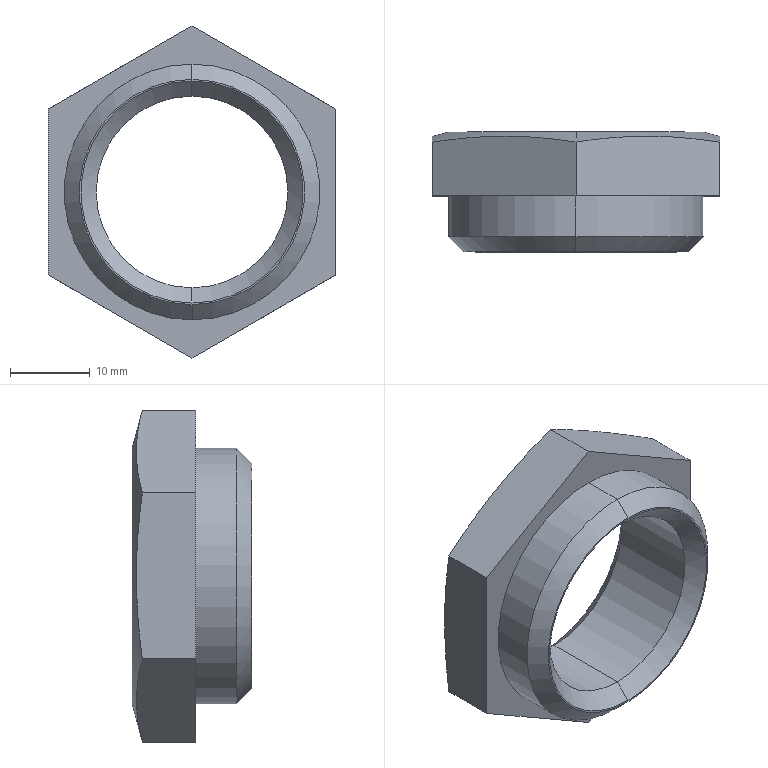Part | SolidWorks | features Boss 1, RevCut 1, Revolution 1 | 1 solid | 21 faces | box 36 x 15 x 41.569 mm | volume 7224 mm3 | plane 9 | cone 8 | cylinder 4 | commonest cylinder face diameters 24 x2 32 x2
STEP:
#1=CARTESIAN_POINT('',(0.,13.1,-12.));
#2=VERTEX_POINT('',#1);
#3=CARTESIAN_POINT('',(0.,13.1,12.));
#4=VERTEX_POINT('',#3);
#5=CARTESIAN_POINT('',(0.,13.1,0.));
#6=DIRECTION('',(0.,1.,0.));
#7=DIRECTION('',(0.,0.,1.));
#8=AXIS2_PLACEMENT_3D('',#5,#6,#7);
#9=CIRCLE('',#8,12.);
#10=EDGE_CURVE('',#2,#4,#9,.T.);
#11=ORIENTED_EDGE('',*,*,#10,.F.);
#12=CARTESIAN_POINT('',(0.,15.,-13.9));
#13=VERTEX_POINT('',#12);
#14=CARTESIAN_POINT('',(0.,15.,-13.9));
#15=DIRECTION('',(0.,0.7071,-0.7071));
#16=VECTOR('',#15,1000.);
#17=LINE('',#14,#16);
#18=EDGE_CURVE('',#2,#13,#17,.T.);
#19=ORIENTED_EDGE('',*,*,#18,.T.);
#20=CARTESIAN_POINT('',(0.,15.,13.9));
#21=VERTEX_POINT('',#20);
#22=CARTESIAN_POINT('',(0.,15.,0.));
#23=DIRECTION('',(0.,1.,0.));
#24=DIRECTION('',(0.,0.,1.));
#25=AXIS2_PLACEMENT_3D('',#22,#23,#24);
#26=CIRCLE('',#25,13.9);
#27=EDGE_CURVE('',#13,#21,#26,.T.);
#28=ORIENTED_EDGE('',*,*,#27,.T.);
#29=CARTESIAN_POINT('',(0.,15.,13.9));
#30=DIRECTION('',(0.,0.7071,0.7071));
#31=VECTOR('',#30,1000.);
#32=LINE('',#29,#31);
#33=EDGE_CURVE('',#4,#21,#32,.T.);
#34=ORIENTED_EDGE('',*,*,#33,.F.);
#35=EDGE_LOOP('',(#11,#19,#28,#34));
#36=FACE_OUTER_BOUND('',#35,.T.);
#37=CARTESIAN_POINT('',(0.,15.,0.));
#38=DIRECTION('',(0.,1.,0.));
#39=DIRECTION('',(0.,0.,1.));
#40=AXIS2_PLACEMENT_3D('',#37,#38,#39);
#41=CONICAL_SURFACE('',#40,13.9,0.7854);
#42=ADVANCED_FACE('',(#36),#41,.F.);
#43=CARTESIAN_POINT('',(0.,15.,16.));
#44=VERTEX_POINT('',#43);
#45=CARTESIAN_POINT('',(0.,15.,-16.));
#46=VERTEX_POINT('',#45);
#47=CARTESIAN_POINT('',(0.,15.,0.));
#48=DIRECTION('',(0.,1.,0.));
#49=DIRECTION('',(0.,0.,1.));
#50=AXIS2_PLACEMENT_3D('',#47,#48,#49);
#51=CIRCLE('',#50,16.);
#52=EDGE_CURVE('',#44,#46,#51,.T.);
#53=ORIENTED_EDGE('',*,*,#52,.F.);
#54=CARTESIAN_POINT('',(0.,13.718,20.785));
#55=VERTEX_POINT('',#54);
#56=CARTESIAN_POINT('',(0.,11.276,29.9));
#57=DIRECTION('',(0.,-0.2588,0.9659));
#58=VECTOR('',#57,1000.);
#59=LINE('',#56,#58);
#60=EDGE_CURVE('',#44,#55,#59,.T.);
#61=ORIENTED_EDGE('',*,*,#60,.T.);
#62=CARTESIAN_POINT('',(18.,13.718,10.392));
#63=VERTEX_POINT('',#62);
#64=CARTESIAN_POINT('',(0.,13.718,20.785));
#65=CARTESIAN_POINT('',(1.5,13.95,19.919));
#66=CARTESIAN_POINT('',(3.,14.138,19.053));
#67=CARTESIAN_POINT('',(6.,14.396,17.321));
#68=CARTESIAN_POINT('',(9.,14.532,15.588));
#69=CARTESIAN_POINT('',(12.,14.396,13.856));
#70=CARTESIAN_POINT('',(15.,14.138,12.124));
#71=CARTESIAN_POINT('',(16.5,13.95,11.258));
#72=CARTESIAN_POINT('',(18.,13.718,10.392));
#73=B_SPLINE_CURVE_WITH_KNOTS('',3,(#64,#65,#66,#67,#68,#69,#70,#71,#72),.UNSPECIFIED.,.F.,.F.,(4,2,1,2,4),(0.000000231,0.005196,0.01039,0.01559,0.02078),.UNSPECIFIED.);
#74=EDGE_CURVE('',#55,#63,#73,.T.);
#75=ORIENTED_EDGE('',*,*,#74,.T.);
#76=CARTESIAN_POINT('',(18.,13.718,-10.392));
#77=VERTEX_POINT('',#76);
#78=CARTESIAN_POINT('',(18.,13.718,10.392));
#79=CARTESIAN_POINT('',(18.,13.949,8.666));
#80=CARTESIAN_POINT('',(18.,14.137,6.939));
#81=CARTESIAN_POINT('',(18.,14.395,3.481));
#82=CARTESIAN_POINT('',(18.,14.464,1.75));
#83=CARTESIAN_POINT('',(18.,14.465,-1.715));
#84=CARTESIAN_POINT('',(18.,14.397,-3.449));
#85=CARTESIAN_POINT('',(18.,14.139,-6.922));
#86=CARTESIAN_POINT('',(18.,13.95,-8.662));
#87=CARTESIAN_POINT('',(18.,13.718,-10.392));
#88=B_SPLINE_CURVE_WITH_KNOTS('',3,(#78,#79,#80,#81,#82,#83,#84,#85,#86,#87),.UNSPECIFIED.,.F.,.F.,(4,2,2,2,4),(0.04105,0.04627,0.05149,0.05671,0.06193),.UNSPECIFIED.);
#89=EDGE_CURVE('',#63,#77,#88,.T.);
#90=ORIENTED_EDGE('',*,*,#89,.T.);
#91=CARTESIAN_POINT('',(0.,13.718,-20.785));
#92=VERTEX_POINT('',#91);
#93=CARTESIAN_POINT('',(18.,13.718,-10.392));
#94=CARTESIAN_POINT('',(16.5,13.95,-11.258));
#95=CARTESIAN_POINT('',(15.,14.138,-12.124));
#96=CARTESIAN_POINT('',(12.,14.396,-13.856));
#97=CARTESIAN_POINT('',(9.,14.532,-15.588));
#98=CARTESIAN_POINT('',(6.,14.396,-17.321));
#99=CARTESIAN_POINT('',(3.,14.138,-19.053));
#100=CARTESIAN_POINT('',(1.5,13.95,-19.919));
#101=CARTESIAN_POINT('',(0.,13.718,-20.785));
#102=B_SPLINE_CURVE_WITH_KNOTS('',3,(#93,#94,#95,#96,#97,#98,#99,#100,#101),.UNSPECIFIED.,.F.,.F.,(4,2,1,2,4),(0.000000231,0.005196,0.01039,0.01559,0.02078),.UNSPECIFIED.);
#103=EDGE_CURVE('',#77,#92,#102,.T.);
#104=ORIENTED_EDGE('',*,*,#103,.T.);
#105=CARTESIAN_POINT('',(0.,11.276,-29.9));
#106=DIRECTION('',(0.,-0.2588,-0.9659));
#107=VECTOR('',#106,1000.);
#108=LINE('',#105,#107);
#109=EDGE_CURVE('',#46,#92,#108,.T.);
#110=ORIENTED_EDGE('',*,*,#109,.F.);
#111=EDGE_LOOP('',(#53,#61,#75,#90,#104,#110));
#112=FACE_OUTER_BOUND('',#111,.T.);
#113=CARTESIAN_POINT('',(0.,11.276,0.));
#114=DIRECTION('',(0.,-1.,0.));
#115=DIRECTION('',(0.,0.,-1.));
#116=AXIS2_PLACEMENT_3D('',#113,#114,#115);
#117=CONICAL_SURFACE('',#116,29.9,1.309);
#118=ADVANCED_FACE('',(#112),#117,.T.);
#119=CARTESIAN_POINT('',(0.,1.9,-12.));
#120=VERTEX_POINT('',#119);
#121=CARTESIAN_POINT('',(0.,1.9,12.));
#122=VERTEX_POINT('',#121);
#123=CARTESIAN_POINT('',(0.,1.9,0.));
#124=DIRECTION('',(0.,1.,0.));
#125=DIRECTION('',(0.,0.,1.));
#126=AXIS2_PLACEMENT_3D('',#123,#124,#125);
#127=CIRCLE('',#126,12.);
#128=EDGE_CURVE('',#120,#122,#127,.T.);
#129=ORIENTED_EDGE('',*,*,#128,.F.);
#130=CARTESIAN_POINT('',(0.,0.,-12.));
#131=DIRECTION('',(0.,1.,0.));
#132=VECTOR('',#131,1000.);
#133=LINE('',#130,#132);
#134=EDGE_CURVE('',#120,#2,#133,.T.);
#135=ORIENTED_EDGE('',*,*,#134,.T.);
#136=ORIENTED_EDGE('',*,*,#10,.T.);
#137=CARTESIAN_POINT('',(0.,0.,12.));
#138=DIRECTION('',(0.,1.,0.));
#139=VECTOR('',#138,1000.);
#140=LINE('',#137,#139);
#141=EDGE_CURVE('',#122,#4,#140,.T.);
#142=ORIENTED_EDGE('',*,*,#141,.F.);
#143=EDGE_LOOP('',(#129,#135,#136,#142));
#144=FACE_OUTER_BOUND('',#143,.T.);
#145=CARTESIAN_POINT('',(0.,0.,0.));
#146=DIRECTION('',(0.,1.,0.));
#147=DIRECTION('',(0.,0.,1.));
#148=AXIS2_PLACEMENT_3D('',#145,#146,#147);
#149=CYLINDRICAL_SURFACE('',#148,12.);
#150=ADVANCED_FACE('',(#144),#149,.F.);
#151=CARTESIAN_POINT('',(0.,1.9,16.));
#152=VERTEX_POINT('',#151);
#153=CARTESIAN_POINT('',(0.,1.9,-16.));
#154=VERTEX_POINT('',#153);
#155=CARTESIAN_POINT('',(0.,1.9,0.));
#156=DIRECTION('',(0.,1.,0.));
#157=DIRECTION('',(0.,0.,1.));
#158=AXIS2_PLACEMENT_3D('',#155,#156,#157);
#159=CIRCLE('',#158,16.);
#160=EDGE_CURVE('',#152,#154,#159,.T.);
#161=ORIENTED_EDGE('',*,*,#160,.T.);
#162=CARTESIAN_POINT('',(0.,7.,-16.));
#163=VERTEX_POINT('',#162);
#164=CARTESIAN_POINT('',(0.,0.,-16.));
#165=DIRECTION('',(0.,1.,0.));
#166=VECTOR('',#165,1000.);
#167=LINE('',#164,#166);
#168=EDGE_CURVE('',#154,#163,#167,.T.);
#169=ORIENTED_EDGE('',*,*,#168,.T.);
#170=CARTESIAN_POINT('',(0.,7.,16.));
#171=VERTEX_POINT('',#170);
#172=CARTESIAN_POINT('',(0.,7.,0.));
#173=DIRECTION('',(0.,1.,0.));
#174=DIRECTION('',(0.,0.,1.));
#175=AXIS2_PLACEMENT_3D('',#172,#173,#174);
#176=CIRCLE('',#175,16.);
#177=EDGE_CURVE('',#171,#163,#176,.T.);
#178=ORIENTED_EDGE('',*,*,#177,.F.);
#179=CARTESIAN_POINT('',(0.,0.,16.));
#180=DIRECTION('',(0.,1.,0.));
#181=VECTOR('',#180,1000.);
#182=LINE('',#179,#181);
#183=EDGE_CURVE('',#152,#171,#182,.T.);
#184=ORIENTED_EDGE('',*,*,#183,.F.);
#185=EDGE_LOOP('',(#161,#169,#178,#184));
#186=FACE_OUTER_BOUND('',#185,.T.);
#187=CARTESIAN_POINT('',(0.,0.,0.));
#188=DIRECTION('',(0.,1.,0.));
#189=DIRECTION('',(0.,0.,1.));
#190=AXIS2_PLACEMENT_3D('',#187,#188,#189);
#191=CYLINDRICAL_SURFACE('',#190,16.);
#192=ADVANCED_FACE('',(#186),#191,.T.);
#193=CARTESIAN_POINT('',(0.,0.,14.1));
#194=VERTEX_POINT('',#193);
#195=CARTESIAN_POINT('',(0.,0.,-14.1));
#196=VERTEX_POINT('',#195);
#197=CARTESIAN_POINT('',(0.,0.,0.));
#198=DIRECTION('',(0.,1.,0.));
#199=DIRECTION('',(0.,0.,1.));
#200=AXIS2_PLACEMENT_3D('',#197,#198,#199);
#201=CIRCLE('',#200,14.1);
#202=EDGE_CURVE('',#194,#196,#201,.T.);
#203=ORIENTED_EDGE('',*,*,#202,.T.);
#204=CARTESIAN_POINT('',(0.,1.9,-16.));
#205=DIRECTION('',(0.,0.7071,-0.7071));
#206=VECTOR('',#205,1000.);
#207=LINE('',#204,#206);
#208=EDGE_CURVE('',#196,#154,#207,.T.);
#209=ORIENTED_EDGE('',*,*,#208,.T.);
#210=ORIENTED_EDGE('',*,*,#160,.F.);
#211=CARTESIAN_POINT('',(0.,1.9,16.));
#212=DIRECTION('',(0.,0.7071,0.7071));
#213=VECTOR('',#212,1000.);
#214=LINE('',#211,#213);
#215=EDGE_CURVE('',#194,#152,#214,.T.);
#216=ORIENTED_EDGE('',*,*,#215,.F.);
#217=EDGE_LOOP('',(#203,#209,#210,#216));
#218=FACE_OUTER_BOUND('',#217,.T.);
#219=CARTESIAN_POINT('',(0.,1.9,0.));
#220=DIRECTION('',(0.,1.,0.));
#221=DIRECTION('',(0.,0.,1.));
#222=AXIS2_PLACEMENT_3D('',#219,#220,#221);
#223=CONICAL_SURFACE('',#222,16.,0.7854);
#224=ADVANCED_FACE('',(#218),#223,.T.);
#225=ORIENTED_EDGE('',*,*,#128,.T.);
#226=CARTESIAN_POINT('',(0.,0.,13.9));
#227=VERTEX_POINT('',#226);
#228=CARTESIAN_POINT('',(0.,0.,13.9));
#229=DIRECTION('',(0.,-0.7071,0.7071));
#230=VECTOR('',#229,1000.);
#231=LINE('',#228,#230);
#232=EDGE_CURVE('',#122,#227,#231,.T.);
#233=ORIENTED_EDGE('',*,*,#232,.T.);
#234=CARTESIAN_POINT('',(0.,0.,-13.9));
#235=VERTEX_POINT('',#234);
#236=CARTESIAN_POINT('',(0.,0.,0.));
#237=DIRECTION('',(0.,1.,0.));
#238=DIRECTION('',(0.,0.,1.));
#239=AXIS2_PLACEMENT_3D('',#236,#237,#238);
#240=CIRCLE('',#239,13.9);
#241=EDGE_CURVE('',#235,#227,#240,.T.);
#242=ORIENTED_EDGE('',*,*,#241,.F.);
#243=CARTESIAN_POINT('',(0.,0.,-13.9));
#244=DIRECTION('',(0.,-0.7071,-0.7071));
#245=VECTOR('',#244,1000.);
#246=LINE('',#243,#245);
#247=EDGE_CURVE('',#120,#235,#246,.T.);
#248=ORIENTED_EDGE('',*,*,#247,.F.);
#249=EDGE_LOOP('',(#225,#233,#242,#248));
#250=FACE_OUTER_BOUND('',#249,.T.);
#251=CARTESIAN_POINT('',(0.,0.,0.));
#252=DIRECTION('',(0.,-1.,0.));
#253=DIRECTION('',(0.,0.,-1.));
#254=AXIS2_PLACEMENT_3D('',#251,#252,#253);
#255=CONICAL_SURFACE('',#254,13.9,0.7854);
#256=ADVANCED_FACE('',(#250),#255,.F.);
#257=ORIENTED_EDGE('',*,*,#232,.F.);
#258=CARTESIAN_POINT('',(0.,1.9,0.));
#259=DIRECTION('',(0.,1.,0.));
#260=DIRECTION('',(0.,0.,1.));
#261=AXIS2_PLACEMENT_3D('',#258,#259,#260);
#262=CIRCLE('',#261,12.);
#263=EDGE_CURVE('',#122,#120,#262,.T.);
#264=ORIENTED_EDGE('',*,*,#263,.T.);
#265=ORIENTED_EDGE('',*,*,#247,.T.);
#266=CARTESIAN_POINT('',(0.,0.,0.));
#267=DIRECTION('',(0.,1.,0.));
#268=DIRECTION('',(0.,0.,1.));
#269=AXIS2_PLACEMENT_3D('',#266,#267,#268);
#270=CIRCLE('',#269,13.9);
#271=EDGE_CURVE('',#227,#235,#270,.T.);
#272=ORIENTED_EDGE('',*,*,#271,.F.);
#273=EDGE_LOOP('',(#257,#264,#265,#272));
#274=FACE_OUTER_BOUND('',#273,.T.);
#275=CARTESIAN_POINT('',(0.,0.,0.));
#276=DIRECTION('',(0.,-1.,0.));
#277=DIRECTION('',(0.,0.,-1.));
#278=AXIS2_PLACEMENT_3D('',#275,#276,#277);
#279=CONICAL_SURFACE('',#278,13.9,0.7854);
#280=ADVANCED_FACE('',(#274),#279,.F.);
#281=ORIENTED_EDGE('',*,*,#241,.T.);
#282=ORIENTED_EDGE('',*,*,#271,.T.);
#283=EDGE_LOOP('',(#281,#282));
#284=FACE_BOUND('',#283,.T.);
#285=ORIENTED_EDGE('',*,*,#202,.F.);
#286=CARTESIAN_POINT('',(0.,0.,0.));
#287=DIRECTION('',(0.,1.,0.));
#288=DIRECTION('',(0.,0.,1.));
#289=AXIS2_PLACEMENT_3D('',#286,#287,#288);
#290=CIRCLE('',#289,14.1);
#291=EDGE_CURVE('',#196,#194,#290,.T.);
#292=ORIENTED_EDGE('',*,*,#291,.F.);
#293=EDGE_LOOP('',(#285,#292));
#294=FACE_OUTER_BOUND('',#293,.T.);
#295=CARTESIAN_POINT('',(-13.9,0.,0.));
#296=DIRECTION('',(0.,-1.,0.));
#297=DIRECTION('',(0.,0.,-1.));
#298=AXIS2_PLACEMENT_3D('',#295,#296,#297);
#299=PLANE('',#298);
#300=ADVANCED_FACE('',(#284,#294),#299,.T.);
#301=ORIENTED_EDGE('',*,*,#208,.F.);
#302=ORIENTED_EDGE('',*,*,#291,.T.);
#303=ORIENTED_EDGE('',*,*,#215,.T.);
#304=CARTESIAN_POINT('',(0.,1.9,0.));
#305=DIRECTION('',(0.,1.,0.));
#306=DIRECTION('',(0.,0.,1.));
#307=AXIS2_PLACEMENT_3D('',#304,#305,#306);
#308=CIRCLE('',#307,16.);
#309=EDGE_CURVE('',#154,#152,#308,.T.);
#310=ORIENTED_EDGE('',*,*,#309,.F.);
#311=EDGE_LOOP('',(#301,#302,#303,#310));
#312=FACE_OUTER_BOUND('',#311,.T.);
#313=CARTESIAN_POINT('',(0.,1.9,0.));
#314=DIRECTION('',(0.,1.,0.));
#315=DIRECTION('',(0.,0.,1.));
#316=AXIS2_PLACEMENT_3D('',#313,#314,#315);
#317=CONICAL_SURFACE('',#316,16.,0.7854);
#318=ADVANCED_FACE('',(#312),#317,.T.);
#319=ORIENTED_EDGE('',*,*,#168,.F.);
#320=ORIENTED_EDGE('',*,*,#309,.T.);
#321=ORIENTED_EDGE('',*,*,#183,.T.);
#322=CARTESIAN_POINT('',(0.,7.,0.));
#323=DIRECTION('',(0.,1.,0.));
#324=DIRECTION('',(0.,0.,1.));
#325=AXIS2_PLACEMENT_3D('',#322,#323,#324);
#326=CIRCLE('',#325,16.);
#327=EDGE_CURVE('',#163,#171,#326,.T.);
#328=ORIENTED_EDGE('',*,*,#327,.F.);
#329=EDGE_LOOP('',(#319,#320,#321,#328));
#330=FACE_OUTER_BOUND('',#329,.T.);
#331=CARTESIAN_POINT('',(0.,0.,0.));
#332=DIRECTION('',(0.,1.,0.));
#333=DIRECTION('',(0.,0.,1.));
#334=AXIS2_PLACEMENT_3D('',#331,#332,#333);
#335=CYLINDRICAL_SURFACE('',#334,16.);
#336=ADVANCED_FACE('',(#330),#335,.T.);
#337=ORIENTED_EDGE('',*,*,#177,.T.);
#338=ORIENTED_EDGE('',*,*,#327,.T.);
#339=EDGE_LOOP('',(#337,#338));
#340=FACE_BOUND('',#339,.T.);
#341=CARTESIAN_POINT('',(18.,7.,10.392));
#342=VERTEX_POINT('',#341);
#343=CARTESIAN_POINT('',(18.,7.,-10.392));
#344=VERTEX_POINT('',#343);
#345=CARTESIAN_POINT('',(18.,7.,10.392));
#346=DIRECTION('',(0.,0.,-1.));
#347=VECTOR('',#346,1000.);
#348=LINE('',#345,#347);
#349=EDGE_CURVE('',#342,#344,#348,.T.);
#350=ORIENTED_EDGE('',*,*,#349,.F.);
#351=CARTESIAN_POINT('',(0.,7.,20.785));
#352=VERTEX_POINT('',#351);
#353=CARTESIAN_POINT('',(0.,7.,20.785));
#354=DIRECTION('',(0.866,0.,-0.5));
#355=VECTOR('',#354,1000.);
#356=LINE('',#353,#355);
#357=EDGE_CURVE('',#352,#342,#356,.T.);
#358=ORIENTED_EDGE('',*,*,#357,.F.);
#359=CARTESIAN_POINT('',(-18.,7.,10.392));
#360=VERTEX_POINT('',#359);
#361=CARTESIAN_POINT('',(-18.,7.,10.392));
#362=DIRECTION('',(0.866,0.,0.5));
#363=VECTOR('',#362,1000.);
#364=LINE('',#361,#363);
#365=EDGE_CURVE('',#360,#352,#364,.T.);
#366=ORIENTED_EDGE('',*,*,#365,.F.);
#367=CARTESIAN_POINT('',(-18.,7.,-10.392));
#368=VERTEX_POINT('',#367);
#369=CARTESIAN_POINT('',(-18.,7.,-10.392));
#370=DIRECTION('',(0.,0.,1.));
#371=VECTOR('',#370,1000.);
#372=LINE('',#369,#371);
#373=EDGE_CURVE('',#368,#360,#372,.T.);
#374=ORIENTED_EDGE('',*,*,#373,.F.);
#375=CARTESIAN_POINT('',(0.,7.,-20.785));
#376=VERTEX_POINT('',#375);
#377=CARTESIAN_POINT('',(0.,7.,-20.785));
#378=DIRECTION('',(-0.866,0.,0.5));
#379=VECTOR('',#378,1000.);
#380=LINE('',#377,#379);
#381=EDGE_CURVE('',#376,#368,#380,.T.);
#382=ORIENTED_EDGE('',*,*,#381,.F.);
#383=CARTESIAN_POINT('',(18.,7.,-10.392));
#384=DIRECTION('',(-0.866,0.,-0.5));
#385=VECTOR('',#384,1000.);
#386=LINE('',#383,#385);
#387=EDGE_CURVE('',#344,#376,#386,.T.);
#388=ORIENTED_EDGE('',*,*,#387,.F.);
#389=EDGE_LOOP('',(#350,#358,#366,#374,#382,#388));
#390=FACE_OUTER_BOUND('',#389,.T.);
#391=CARTESIAN_POINT('',(-16.,7.,0.));
#392=DIRECTION('',(0.,-1.,0.));
#393=DIRECTION('',(0.,0.,-1.));
#394=AXIS2_PLACEMENT_3D('',#391,#392,#393);
#395=PLANE('',#394);
#396=ADVANCED_FACE('',(#340,#390),#395,.T.);
#397=ORIENTED_EDGE('',*,*,#134,.F.);
#398=ORIENTED_EDGE('',*,*,#263,.F.);
#399=ORIENTED_EDGE('',*,*,#141,.T.);
#400=CARTESIAN_POINT('',(0.,13.1,0.));
#401=DIRECTION('',(0.,1.,0.));
#402=DIRECTION('',(0.,0.,1.));
#403=AXIS2_PLACEMENT_3D('',#400,#401,#402);
#404=CIRCLE('',#403,12.);
#405=EDGE_CURVE('',#4,#2,#404,.T.);
#406=ORIENTED_EDGE('',*,*,#405,.T.);
#407=EDGE_LOOP('',(#397,#398,#399,#406));
#408=FACE_OUTER_BOUND('',#407,.T.);
#409=CARTESIAN_POINT('',(0.,0.,0.));
#410=DIRECTION('',(0.,1.,0.));
#411=DIRECTION('',(0.,0.,1.));
#412=AXIS2_PLACEMENT_3D('',#409,#410,#411);
#413=CYLINDRICAL_SURFACE('',#412,12.);
#414=ADVANCED_FACE('',(#408),#413,.F.);
#415=ORIENTED_EDGE('',*,*,#74,.F.);
#416=CARTESIAN_POINT('',(0.,7.,20.785));
#417=DIRECTION('',(0.,1.,0.));
#418=VECTOR('',#417,1000.);
#419=LINE('',#416,#418);
#420=EDGE_CURVE('',#352,#55,#419,.T.);
#421=ORIENTED_EDGE('',*,*,#420,.F.);
#422=ORIENTED_EDGE('',*,*,#357,.T.);
#423=CARTESIAN_POINT('',(18.,7.,10.392));
#424=DIRECTION('',(0.,1.,0.));
#425=VECTOR('',#424,1000.);
#426=LINE('',#423,#425);
#427=EDGE_CURVE('',#342,#63,#426,.T.);
#428=ORIENTED_EDGE('',*,*,#427,.T.);
#429=EDGE_LOOP('',(#415,#421,#422,#428));
#430=FACE_OUTER_BOUND('',#429,.T.);
#431=CARTESIAN_POINT('',(0.,7.,20.785));
#432=DIRECTION('',(0.5,0.,0.866));
#433=DIRECTION('',(0.866,0.,-0.5));
#434=AXIS2_PLACEMENT_3D('',#431,#432,#433);
#435=PLANE('',#434);
#436=ADVANCED_FACE('',(#430),#435,.T.);
#437=CARTESIAN_POINT('',(-18.,13.718,10.392));
#438=VERTEX_POINT('',#437);
#439=CARTESIAN_POINT('',(-18.,13.718,10.392));
#440=CARTESIAN_POINT('',(-16.5,13.95,11.258));
#441=CARTESIAN_POINT('',(-15.,14.138,12.124));
#442=CARTESIAN_POINT('',(-12.,14.396,13.856));
#443=CARTESIAN_POINT('',(-9.,14.532,15.588));
#444=CARTESIAN_POINT('',(-6.,14.396,17.321));
#445=CARTESIAN_POINT('',(-3.,14.138,19.053));
#446=CARTESIAN_POINT('',(-1.5,13.95,19.919));
#447=CARTESIAN_POINT('',(0.,13.718,20.785));
#448=B_SPLINE_CURVE_WITH_KNOTS('',3,(#439,#440,#441,#442,#443,#444,#445,#446,#447),.UNSPECIFIED.,.F.,.F.,(4,2,1,2,4),(0.000000231,0.005196,0.01039,0.01559,0.02078),.UNSPECIFIED.);
#449=EDGE_CURVE('',#438,#55,#448,.T.);
#450=ORIENTED_EDGE('',*,*,#449,.F.);
#451=CARTESIAN_POINT('',(-18.,7.,10.392));
#452=DIRECTION('',(0.,1.,0.));
#453=VECTOR('',#452,1000.);
#454=LINE('',#451,#453);
#455=EDGE_CURVE('',#360,#438,#454,.T.);
#456=ORIENTED_EDGE('',*,*,#455,.F.);
#457=ORIENTED_EDGE('',*,*,#365,.T.);
#458=ORIENTED_EDGE('',*,*,#420,.T.);
#459=EDGE_LOOP('',(#450,#456,#457,#458));
#460=FACE_OUTER_BOUND('',#459,.T.);
#461=CARTESIAN_POINT('',(-18.,7.,10.392));
#462=DIRECTION('',(-0.5,0.,0.866));
#463=DIRECTION('',(0.866,0.,0.5));
#464=AXIS2_PLACEMENT_3D('',#461,#462,#463);
#465=PLANE('',#464);
#466=ADVANCED_FACE('',(#460),#465,.T.);
#467=CARTESIAN_POINT('',(-18.,13.718,-10.392));
#468=VERTEX_POINT('',#467);
#469=CARTESIAN_POINT('',(-18.,13.718,-10.392));
#470=CARTESIAN_POINT('',(-18.,13.95,-8.662));
#471=CARTESIAN_POINT('',(-18.,14.139,-6.922));
#472=CARTESIAN_POINT('',(-18.,14.397,-3.449));
#473=CARTESIAN_POINT('',(-18.,14.465,-1.715));
#474=CARTESIAN_POINT('',(-18.,14.464,1.75));
#475=CARTESIAN_POINT('',(-18.,14.395,3.481));
#476=CARTESIAN_POINT('',(-18.,14.137,6.939));
#477=CARTESIAN_POINT('',(-18.,13.949,8.666));
#478=CARTESIAN_POINT('',(-18.,13.718,10.392));
#479=B_SPLINE_CURVE_WITH_KNOTS('',3,(#469,#470,#471,#472,#473,#474,#475,#476,#477,#478),.UNSPECIFIED.,.F.,.F.,(4,2,2,2,4),(0.01753,0.02276,0.02799,0.03322,0.03845),.UNSPECIFIED.);
#480=EDGE_CURVE('',#468,#438,#479,.T.);
#481=ORIENTED_EDGE('',*,*,#480,.F.);
#482=CARTESIAN_POINT('',(-18.,7.,-10.392));
#483=DIRECTION('',(0.,1.,0.));
#484=VECTOR('',#483,1000.);
#485=LINE('',#482,#484);
#486=EDGE_CURVE('',#368,#468,#485,.T.);
#487=ORIENTED_EDGE('',*,*,#486,.F.);
#488=ORIENTED_EDGE('',*,*,#373,.T.);
#489=ORIENTED_EDGE('',*,*,#455,.T.);
#490=EDGE_LOOP('',(#481,#487,#488,#489));
#491=FACE_OUTER_BOUND('',#490,.T.);
#492=CARTESIAN_POINT('',(-18.,7.,-10.392));
#493=DIRECTION('',(-1.,0.,0.));
#494=DIRECTION('',(0.,0.,1.));
#495=AXIS2_PLACEMENT_3D('',#492,#493,#494);
#496=PLANE('',#495);
#497=ADVANCED_FACE('',(#491),#496,.T.);
#498=CARTESIAN_POINT('',(0.,13.718,-20.785));
#499=CARTESIAN_POINT('',(-1.5,13.95,-19.919));
#500=CARTESIAN_POINT('',(-3.,14.138,-19.053));
#501=CARTESIAN_POINT('',(-6.,14.396,-17.321));
#502=CARTESIAN_POINT('',(-9.,14.532,-15.588));
#503=CARTESIAN_POINT('',(-12.,14.396,-13.856));
#504=CARTESIAN_POINT('',(-15.,14.138,-12.124));
#505=CARTESIAN_POINT('',(-16.5,13.95,-11.258));
#506=CARTESIAN_POINT('',(-18.,13.718,-10.392));
#507=B_SPLINE_CURVE_WITH_KNOTS('',3,(#498,#499,#500,#501,#502,#503,#504,#505,#506),.UNSPECIFIED.,.F.,.F.,(4,2,1,2,4),(0.000000231,0.005196,0.01039,0.01559,0.02078),.UNSPECIFIED.);
#508=EDGE_CURVE('',#92,#468,#507,.T.);
#509=ORIENTED_EDGE('',*,*,#508,.F.);
#510=CARTESIAN_POINT('',(0.,7.,-20.785));
#511=DIRECTION('',(0.,1.,0.));
#512=VECTOR('',#511,1000.);
#513=LINE('',#510,#512);
#514=EDGE_CURVE('',#376,#92,#513,.T.);
#515=ORIENTED_EDGE('',*,*,#514,.F.);
#516=ORIENTED_EDGE('',*,*,#381,.T.);
#517=ORIENTED_EDGE('',*,*,#486,.T.);
#518=EDGE_LOOP('',(#509,#515,#516,#517));
#519=FACE_OUTER_BOUND('',#518,.T.);
#520=CARTESIAN_POINT('',(0.,7.,-20.785));
#521=DIRECTION('',(-0.5,0.,-0.866));
#522=DIRECTION('',(-0.866,0.,0.5));
#523=AXIS2_PLACEMENT_3D('',#520,#521,#522);
#524=PLANE('',#523);
#525=ADVANCED_FACE('',(#519),#524,.T.);
#526=ORIENTED_EDGE('',*,*,#103,.F.);
#527=CARTESIAN_POINT('',(18.,7.,-10.392));
#528=DIRECTION('',(0.,1.,0.));
#529=VECTOR('',#528,1000.);
#530=LINE('',#527,#529);
#531=EDGE_CURVE('',#344,#77,#530,.T.);
#532=ORIENTED_EDGE('',*,*,#531,.F.);
#533=ORIENTED_EDGE('',*,*,#387,.T.);
#534=ORIENTED_EDGE('',*,*,#514,.T.);
#535=EDGE_LOOP('',(#526,#532,#533,#534));
#536=FACE_OUTER_BOUND('',#535,.T.);
#537=CARTESIAN_POINT('',(18.,7.,-10.392));
#538=DIRECTION('',(0.5,0.,-0.866));
#539=DIRECTION('',(-0.866,0.,-0.5));
#540=AXIS2_PLACEMENT_3D('',#537,#538,#539);
#541=PLANE('',#540);
#542=ADVANCED_FACE('',(#536),#541,.T.);
#543=ORIENTED_EDGE('',*,*,#89,.F.);
#544=ORIENTED_EDGE('',*,*,#427,.F.);
#545=ORIENTED_EDGE('',*,*,#349,.T.);
#546=ORIENTED_EDGE('',*,*,#531,.T.);
#547=EDGE_LOOP('',(#543,#544,#545,#546));
#548=FACE_OUTER_BOUND('',#547,.T.);
#549=CARTESIAN_POINT('',(18.,7.,10.392));
#550=DIRECTION('',(1.,0.,0.));
#551=DIRECTION('',(0.,0.,-1.));
#552=AXIS2_PLACEMENT_3D('',#549,#550,#551);
#553=PLANE('',#552);
#554=ADVANCED_FACE('',(#548),#553,.T.);
#555=ORIENTED_EDGE('',*,*,#60,.F.);
#556=CARTESIAN_POINT('',(0.,15.,0.));
#557=DIRECTION('',(0.,1.,0.));
#558=DIRECTION('',(0.,0.,1.));
#559=AXIS2_PLACEMENT_3D('',#556,#557,#558);
#560=CIRCLE('',#559,16.);
#561=EDGE_CURVE('',#46,#44,#560,.T.);
#562=ORIENTED_EDGE('',*,*,#561,.F.);
#563=ORIENTED_EDGE('',*,*,#109,.T.);
#564=ORIENTED_EDGE('',*,*,#508,.T.);
#565=ORIENTED_EDGE('',*,*,#480,.T.);
#566=ORIENTED_EDGE('',*,*,#449,.T.);
#567=EDGE_LOOP('',(#555,#562,#563,#564,#565,#566));
#568=FACE_OUTER_BOUND('',#567,.T.);
#569=CARTESIAN_POINT('',(0.,11.276,0.));
#570=DIRECTION('',(0.,-1.,0.));
#571=DIRECTION('',(0.,0.,-1.));
#572=AXIS2_PLACEMENT_3D('',#569,#570,#571);
#573=CONICAL_SURFACE('',#572,29.9,1.309);
#574=ADVANCED_FACE('',(#568),#573,.T.);
#575=CARTESIAN_POINT('',(0.,15.,0.));
#576=DIRECTION('',(0.,1.,0.));
#577=DIRECTION('',(0.,0.,1.));
#578=AXIS2_PLACEMENT_3D('',#575,#576,#577);
#579=CIRCLE('',#578,13.9);
#580=EDGE_CURVE('',#21,#13,#579,.T.);
#581=ORIENTED_EDGE('',*,*,#580,.F.);
#582=ORIENTED_EDGE('',*,*,#27,.F.);
#583=EDGE_LOOP('',(#581,#582));
#584=FACE_BOUND('',#583,.T.);
#585=ORIENTED_EDGE('',*,*,#561,.T.);
#586=ORIENTED_EDGE('',*,*,#52,.T.);
#587=EDGE_LOOP('',(#585,#586));
#588=FACE_OUTER_BOUND('',#587,.T.);
#589=CARTESIAN_POINT('',(-16.,15.,0.));
#590=DIRECTION('',(0.,1.,0.));
#591=DIRECTION('',(0.,0.,1.));
#592=AXIS2_PLACEMENT_3D('',#589,#590,#591);
#593=PLANE('',#592);
#594=ADVANCED_FACE('',(#584,#588),#593,.T.);
#595=ORIENTED_EDGE('',*,*,#18,.F.);
#596=ORIENTED_EDGE('',*,*,#405,.F.);
#597=ORIENTED_EDGE('',*,*,#33,.T.);
#598=ORIENTED_EDGE('',*,*,#580,.T.);
#599=EDGE_LOOP('',(#595,#596,#597,#598));
#600=FACE_OUTER_BOUND('',#599,.T.);
#601=CARTESIAN_POINT('',(0.,15.,0.));
#602=DIRECTION('',(0.,1.,0.));
#603=DIRECTION('',(0.,0.,1.));
#604=AXIS2_PLACEMENT_3D('',#601,#602,#603);
#605=CONICAL_SURFACE('',#604,13.9,0.7854);
#606=ADVANCED_FACE('',(#600),#605,.F.);
#607=CLOSED_SHELL('',(#42,#118,#150,#192,#224,#256,#280,#300,#318,#336,#396,#414,#436,#466,#497,#525,#542,#554,#574,#594,#606));
#608=MANIFOLD_SOLID_BREP('',#607);
#609=CARTESIAN_POINT('',(0.,0.,0.));
#610=DIRECTION('',(0.,0.,1.));
#611=DIRECTION('',(1.,0.,0.));
#612=AXIS2_PLACEMENT_3D('',#609,#610,#611);
#613=(LENGTH_UNIT()NAMED_UNIT(*)SI_UNIT(.MILLI.,.METRE.));
#614=UNCERTAINTY_MEASURE_WITH_UNIT(LENGTH_MEASURE(0.00001),#613,'','');
#615=(NAMED_UNIT(*)PLANE_ANGLE_UNIT()SI_UNIT($,.RADIAN.));
#616=(NAMED_UNIT(*)SI_UNIT($,.STERADIAN.)SOLID_ANGLE_UNIT());
#617=(GEOMETRIC_REPRESENTATION_CONTEXT(3)GLOBAL_UNCERTAINTY_ASSIGNED_CONTEXT((#614))GLOBAL_UNIT_ASSIGNED_CONTEXT((#613,#615,#616))REPRESENTATION_CONTEXT('',''));
#618=ADVANCED_BREP_SHAPE_REPRESENTATION('',(#608,#612),#617);